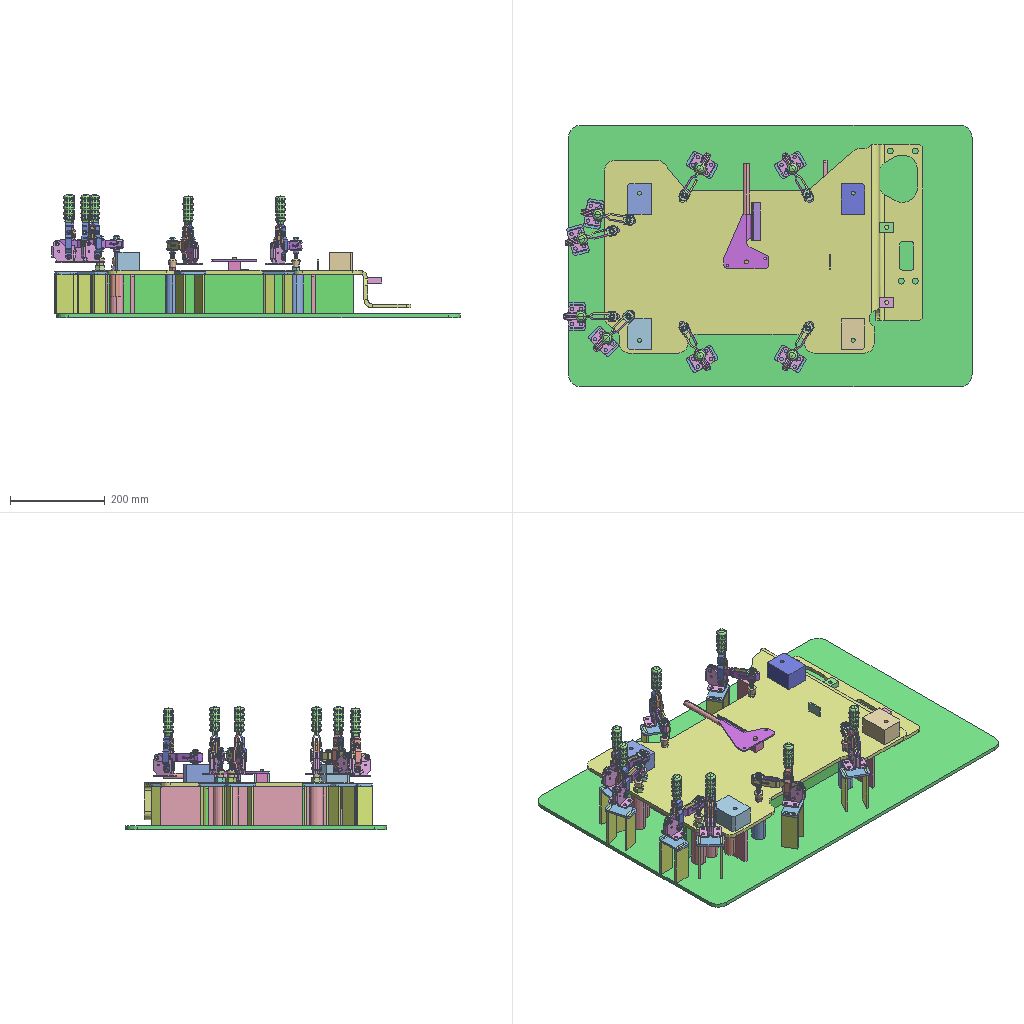Assembly | SolidWorks | 10 different items | 54 placed | box 860 x 550 x 260 mm
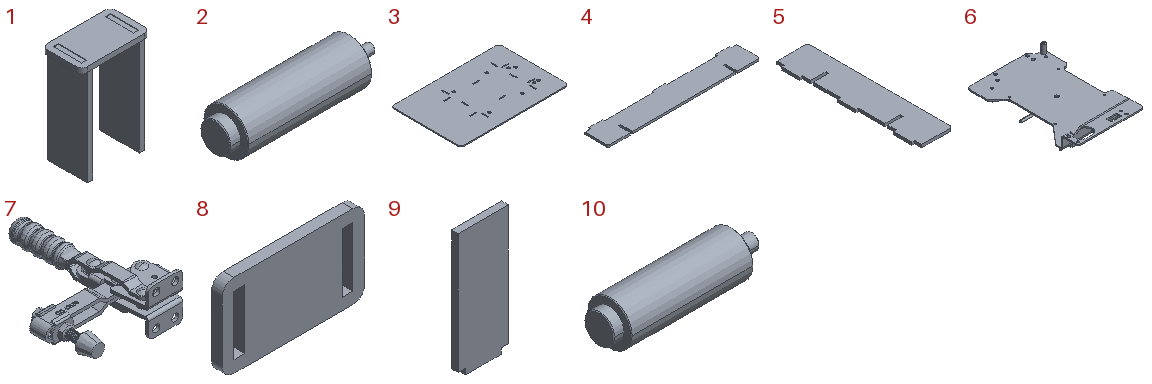Parts list (item | name | quantity | parent item | size | volume | features):
1 | (subassembly) | x8 | - | 60 x 35 x 88.5 mm | 35701 mm3 | features LocalLPattern 1, ReferencePattern 1
2 | - | x4 | - | 104 x 30 x 30 mm | 61439 mm3 | features Chamfer 1, Revolution 1
3 | - | x1 | - | 850 x 550 x 8 mm | 3677202 mm3 | features FlatPattern 1, SMBaseFlange 1, SheetMetal 1
4 | - | x2 | - | 550 x 91 x 8 mm | 372474 mm3 | features FlatPattern 1, SMBaseFlange 1, SheetMetal 1
5 | - | x2 | - | 91 x 400 x 8 mm | 271738 mm3 | features FlatPattern 1, SMBaseFlange 1, SheetMetal 1
6 | - | x1 | - | 440 x 670 x 117 mm | 2554024 mm3 | features BaseBody 20
7 | - | x8 | - | 116.904 x 150.116 x 46 mm | 60512 mm3 | features BaseBody 18
8 | - | x8 | in 1 | 60 x 4.5 x 35 mm | 8341 mm3 | features FlatPattern 1, SMBaseFlange 1, SheetMetal 1
9 | - | x16 | in 1 | 35 x 4.5 x 88 mm | 13680 mm3 | features FlatPattern 1, SMBaseFlange 1, SheetMetal 1
10 | - | x4 | - | 104 x 30 x 30 mm | 62360 mm3 | features Chamfer 1, Revolution 1
Mates (type | each side: item.copy, entity, surface, feature):
In the top assembly
InPlace | 3.1 plane | assembly plane
InPlace | 10.1 plane | assembly plane
Concentric | 6.1 face cylinder 20Y-43-D217B.STEP-1-solid16 | 10.2 face cylinder Revolve1
Coincident | 3.1 face plane Base-Flange1 | 10.2 face plane Revolve1
Concentric | 6.1 face cylinder 20Y-43-D217B.STEP-1-solid7 | 10.3 face cylinder Revolve1
Coincident | 3.1 face plane Base-Flange1 | 10.3 face plane Revolve1
Concentric | 6.1 face cylinder 20Y-43-D217B.STEP-1-solid5 | 10.4 face cylinder Revolve1
Coincident | 3.1 face plane Base-Flange1 | 10.4 face plane Revolve1
Concentric | 6.1 face cylinder 20Y-43-D217B.STEP-1-solid9 | 2.1 face cylinder Revolve1
Coincident | 3.1 face plane Base-Flange1 | 2.1 face plane Revolve1
Concentric | 6.1 face cylinder 20Y-43-D217B.STEP-1-solid18 | 2.2 face cylinder Revolve1
Coincident | 3.1 face plane Base-Flange1 | 2.2 face plane Revolve1
Concentric | 6.1 face cylinder 20Y-43-D217B.STEP-1-solid11 | 2.3 face cylinder Revolve1
Coincident | 3.1 face plane Base-Flange1 | 2.3 face plane Revolve1
Concentric | 6.1 face cylinder 20Y-43-D217B.STEP-1-solid11 | 2.4 face cylinder Revolve1
Coincident | 3.1 face plane Base-Flange1 | 2.4 face plane Revolve1
Concentric | 6.1 face cylinder 20Y-43-D217B.STEP-1-solid9 | 7.1 edge
Coincident | 6.1 face plane 20Y-43-D217B.STEP-1-solid9 | 7.1 face plane
PlanarAngleDim | 7.1 face plane | 6.1 face plane 20Y-43-D217B.STEP-1-solid11
Coincident | 6.1 face plane 20Y-43-D217B.STEP-1-solid16 | 7.2 face plane
Concentric | 6.1 face cylinder 20Y-43-D217B.STEP-1-solid16 | 7.2 edge
Coincident | 6.1 face plane 20Y-43-D217B.STEP-1-solid7 | 7.3 face plane
Concentric | 6.1 face cylinder 20Y-43-D217B.STEP-1-solid7 | 7.3 edge
Perpendicular | 6.1 face plane 20Y-43-D217B.STEP-1-solid11 | 7.2 face plane
PlanarAngleDim | 7.3 face plane | 6.1 face plane 20Y-43-D217B.STEP-1-solid11
Coincident | 6.1 face plane 20Y-43-D217B.STEP-1-solid18 | 7.4 face plane
Concentric | 6.1 face cylinder 20Y-43-D217B.STEP-1-solid18 | 7.4 edge
PlanarAngleDim | 6.1 face plane 20Y-43-D217B.STEP-1-solid11 | 7.4 face plane
Concentric | 6.1 face cylinder 20Y-43-D217B.STEP-1-solid3 | 7.5 edge
Coincident | 6.1 face plane 20Y-43-D217B.STEP-1-solid3 | 7.5 face plane
Concentric | 6.1 face cylinder 20Y-43-D217B.STEP-1-solid5 | 7.6 edge
Coincident | 6.1 face plane 20Y-43-D217B.STEP-1-solid5 | 7.6 face plane
PlanarAngleDim | 7.5 face plane | 6.1 face plane 20Y-43-D217B.STEP-1-solid11
PlanarAngleDim | 7.6 face plane | 6.1 face plane 20Y-43-D217B.STEP-1-solid11
InPlace | 4.1 plane | assembly plane
InPlace | 5.1 plane | assembly plane
Coincident | 3.1 face plane Base-Flange1 | 9.1 face plane Base-Flange1
DistanceDim | 8.1 face plane Base-Flange1 | 7.3 face plane
Coincident | 7.3 edge | 8.1 face plane Base-Flange1
Coincident | 3.1 face plane Base-Flange1 | 9.2 face plane Base-Flange1
Coincident | 7.2 edge | 8.2 face plane Base-Flange1
DistanceDim | 8.2 face plane Base-Flange1 | 7.2 face plane
Coincident | 3.1 face plane Base-Flange1 | 9.3 face plane Base-Flange1
Coincident | 7.5 edge | 8.3 face plane Base-Flange1
DistanceDim | 7.5 face plane | 8.3 face plane Base-Flange1
Coincident | 3.1 face plane Base-Flange1 | 9.4 face plane Base-Flange1
Coincident | 7.6 edge | 8.4 face plane Base-Flange1
DistanceDim | 7.6 face plane | 8.4 face plane Base-Flange1
Coincident | 3.1 face plane Base-Flange1 | 9.5 face plane Base-Flange1
Coincident | 7.7 edge | 8.5 face plane Base-Flange1
DistanceDim | 7.7 face plane | 8.5 face plane Base-Flange1
Coincident | 3.1 face plane Base-Flange1 | 9.6 face plane Base-Flange1
Coincident | 7.8 edge | 8.6 face plane Base-Flange1
DistanceDim | 7.8 face plane | 8.6 face plane Base-Flange1
In subassembly 1
Coincident | 8.7 face plane Base-Flange1 | 9.7 face plane Base-Flange1 | 3 times